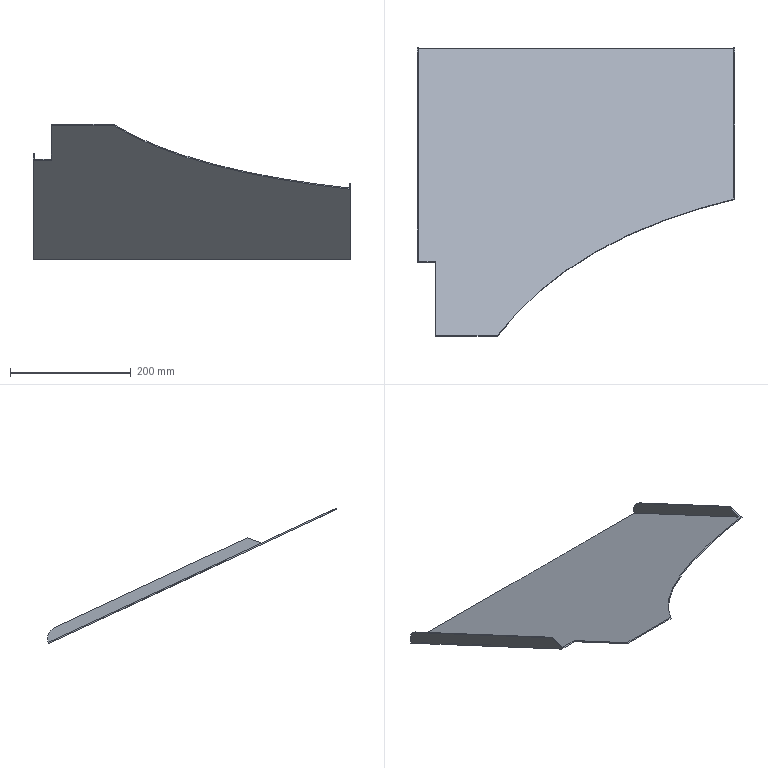Part | NX | features solid 2 | 1 solid | 17 faces | box 525 x 478.276 x 223.963 mm | volume 442323 mm3 | plane 14 | cylinder 2 | spline 1 | commonest cylinder face diameters 40 x2
STEP:
#1=CARTESIAN_POINT('',(-287.,720.,-282.15));
#2=VERTEX_POINT('',#1);
#3=CARTESIAN_POINT('',(-287.,720.,-279.943));
#4=VERTEX_POINT('',#3);
#5=CARTESIAN_POINT('',(-287.,720.,-430.));
#6=DIRECTION('',(0.,0.,1.));
#7=VECTOR('',#6,1000.);
#8=LINE('',#5,#7);
#9=EDGE_CURVE('',#2,#4,#8,.T.);
#10=ORIENTED_EDGE('',*,*,#9,.F.);
#11=CARTESIAN_POINT('',(-808.,720.,-282.15));
#12=VERTEX_POINT('',#11);
#13=CARTESIAN_POINT('',(188.564,720.,-282.15));
#14=DIRECTION('',(-1.,0.,0.));
#15=VECTOR('',#14,1000.);
#16=LINE('',#13,#15);
#17=EDGE_CURVE('',#2,#12,#16,.T.);
#18=ORIENTED_EDGE('',*,*,#17,.T.);
#19=CARTESIAN_POINT('',(-808.,720.,-279.943));
#20=VERTEX_POINT('',#19);
#21=CARTESIAN_POINT('',(-808.,720.,-430.));
#22=DIRECTION('',(0.,0.,-1.));
#23=VECTOR('',#22,1000.);
#24=LINE('',#21,#23);
#25=EDGE_CURVE('',#20,#12,#24,.T.);
#26=ORIENTED_EDGE('',*,*,#25,.F.);
#27=CARTESIAN_POINT('',(188.564,720.,-279.943));
#28=DIRECTION('',(-1.,0.,0.));
#29=VECTOR('',#28,1000.);
#30=LINE('',#27,#29);
#31=EDGE_CURVE('',#4,#20,#30,.T.);
#32=ORIENTED_EDGE('',*,*,#31,.F.);
#33=EDGE_LOOP('',(#10,#18,#26,#32));
#34=FACE_BOUND('',#33,.T.);
#35=CARTESIAN_POINT('',(188.564,720.,-430.));
#36=DIRECTION('',(0.,-1.,0.));
#37=DIRECTION('',(-1.,0.,0.));
#38=AXIS2_PLACEMENT_3D('',#35,#36,#37);
#39=PLANE('',#38);
#40=ADVANCED_FACE('',(#34),#39,.F.);
#41=CARTESIAN_POINT('',(-287.,472.974,-164.753));
#42=VERTEX_POINT('',#41);
#43=CARTESIAN_POINT('',(-285.,472.974,-164.753));
#44=VERTEX_POINT('',#43);
#45=CARTESIAN_POINT('',(-353.018,472.974,-164.753));
#46=DIRECTION('',(-1.,0.,0.));
#47=VECTOR('',#46,1000.);
#48=LINE('',#45,#47);
#49=EDGE_CURVE('',#42,#44,#48,.F.);
#50=ORIENTED_EDGE('',*,*,#49,.F.);
#51=CARTESIAN_POINT('',(-287.,417.055,-138.678));
#52=DIRECTION('',(0.,0.9063,-0.4226));
#53=VECTOR('',#52,1000.);
#54=LINE('',#51,#53);
#55=EDGE_CURVE('',#42,#4,#54,.T.);
#56=ORIENTED_EDGE('',*,*,#55,.T.);
#57=ORIENTED_EDGE('',*,*,#31,.T.);
#58=CARTESIAN_POINT('',(-808.,367.658,-115.644));
#59=VERTEX_POINT('',#58);
#60=CARTESIAN_POINT('',(-808.,417.055,-138.678));
#61=DIRECTION('',(0.,-0.9063,0.4226));
#62=VECTOR('',#61,1000.);
#63=LINE('',#60,#62);
#64=EDGE_CURVE('',#20,#59,#63,.T.);
#65=ORIENTED_EDGE('',*,*,#64,.T.);
#66=CARTESIAN_POINT('',(-780.,367.658,-115.644));
#67=VERTEX_POINT('',#66);
#68=CARTESIAN_POINT('',(-779.,367.658,-115.644));
#69=DIRECTION('',(-1.,0.,0.));
#70=VECTOR('',#69,1000.);
#71=LINE('',#68,#70);
#72=EDGE_CURVE('',#67,#59,#71,.T.);
#73=ORIENTED_EDGE('',*,*,#72,.F.);
#74=CARTESIAN_POINT('',(-780.,244.443,-58.187));
#75=VERTEX_POINT('',#74);
#76=CARTESIAN_POINT('',(-780.,272.567,-71.302));
#77=DIRECTION('',(0.,0.9063,-0.4226));
#78=VECTOR('',#77,1000.);
#79=LINE('',#76,#78);
#80=EDGE_CURVE('',#75,#67,#79,.T.);
#81=ORIENTED_EDGE('',*,*,#80,.F.);
#82=CARTESIAN_POINT('',(-677.72,244.443,-58.187));
#83=VERTEX_POINT('',#82);
#84=CARTESIAN_POINT('',(-353.018,244.443,-58.187));
#85=DIRECTION('',(1.,0.,0.));
#86=VECTOR('',#85,1000.);
#87=LINE('',#84,#86);
#88=EDGE_CURVE('',#75,#83,#87,.T.);
#89=ORIENTED_EDGE('',*,*,#88,.T.);
#90=CARTESIAN_POINT('',(-285.,471.162,-163.908));
#91=VERTEX_POINT('',#90);
#92=CARTESIAN_POINT('',(-677.72,244.443,-58.187));
#93=CARTESIAN_POINT('',(-672.167,251.77,-61.604));
#94=CARTESIAN_POINT('',(-663.423,262.605,-66.657));
#95=CARTESIAN_POINT('',(-650.978,276.698,-73.228));
#96=CARTESIAN_POINT('',(-641.165,287.179,-78.116));
#97=CARTESIAN_POINT('',(-631.216,297.219,-82.798));
#98=CARTESIAN_POINT('',(-620.962,307.004,-87.36));
#99=CARTESIAN_POINT('',(-612.158,314.946,-91.063));
#100=CARTESIAN_POINT('',(-604.955,321.177,-93.969));
#101=CARTESIAN_POINT('',(-600.401,325.008,-95.756));
#102=CARTESIAN_POINT('',(-596.688,328.067,-97.182));
#103=CARTESIAN_POINT('',(-593.065,331.011,-98.555));
#104=CARTESIAN_POINT('',(-586.789,336.01,-100.886));
#105=CARTESIAN_POINT('',(-573.857,345.914,-105.504));
#106=CARTESIAN_POINT('',(-558.47,356.808,-110.584));
#107=CARTESIAN_POINT('',(-542.419,367.323,-115.487));
#108=CARTESIAN_POINT('',(-530.057,375.012,-119.073));
#109=CARTESIAN_POINT('',(-517.377,382.503,-122.566));
#110=CARTESIAN_POINT('',(-506.516,388.595,-125.406));
#111=CARTESIAN_POINT('',(-498.82,392.748,-127.343));
#112=CARTESIAN_POINT('',(-494.304,395.136,-128.457));
#113=CARTESIAN_POINT('',(-490.241,397.26,-129.447));
#114=CARTESIAN_POINT('',(-484.961,399.97,-130.711));
#115=CARTESIAN_POINT('',(-476.523,404.197,-132.682));
#116=CARTESIAN_POINT('',(-465.791,409.379,-135.099));
#117=CARTESIAN_POINT('',(-448.313,417.413,-138.845));
#118=CARTESIAN_POINT('',(-430.339,425.076,-142.418));
#119=CARTESIAN_POINT('',(-411.886,432.361,-145.815));
#120=CARTESIAN_POINT('',(-400.134,436.764,-147.868));
#121=CARTESIAN_POINT('',(-390.645,440.181,-149.462));
#122=CARTESIAN_POINT('',(-383.373,442.729,-150.65));
#123=CARTESIAN_POINT('',(-376.401,445.108,-151.759));
#124=CARTESIAN_POINT('',(-367.079,448.209,-153.205));
#125=CARTESIAN_POINT('',(-357.741,451.192,-154.596));
#126=CARTESIAN_POINT('',(-348.382,454.06,-155.933));
#127=CARTESIAN_POINT('',(-341.353,456.153,-156.91));
#128=CARTESIAN_POINT('',(-335.488,457.849,-157.7));
#129=CARTESIAN_POINT('',(-330.79,459.178,-158.32));
#130=CARTESIAN_POINT('',(-327.855,459.995,-158.701));
#131=CARTESIAN_POINT('',(-325.793,460.562,-158.966));
#132=CARTESIAN_POINT('',(-324.625,460.882,-159.115));
#133=CARTESIAN_POINT('',(-323.869,461.088,-159.211));
#134=CARTESIAN_POINT('',(-323.323,461.236,-159.28));
#135=CARTESIAN_POINT('',(-322.949,461.338,-159.327));
#136=CARTESIAN_POINT('',(-322.199,461.541,-159.422));
#137=CARTESIAN_POINT('',(-320.706,461.943,-159.609));
#138=CARTESIAN_POINT('',(-318.393,462.561,-159.898));
#139=CARTESIAN_POINT('',(-314.394,463.619,-160.391));
#140=CARTESIAN_POINT('',(-308.795,465.082,-161.073));
#141=CARTESIAN_POINT('',(-302.405,466.73,-161.842));
#142=CARTESIAN_POINT('',(-297.517,467.981,-162.425));
#143=CARTESIAN_POINT('',(-294.603,468.725,-162.772));
#144=CARTESIAN_POINT('',(-292.74,469.199,-162.993));
#145=CARTESIAN_POINT('',(-291.2,469.59,-163.175));
#146=CARTESIAN_POINT('',(-290.27,469.826,-163.286));
#147=CARTESIAN_POINT('',(-289.417,470.043,-163.386));
#148=CARTESIAN_POINT('',(-288.93,470.166,-163.444));
#149=CARTESIAN_POINT('',(-287.978,470.408,-163.557));
#150=CARTESIAN_POINT('',(-286.649,470.744,-163.714));
#151=CARTESIAN_POINT('',(-285.552,471.022,-163.843));
#152=CARTESIAN_POINT('',(-285.,471.162,-163.908));
#153=B_SPLINE_CURVE_WITH_KNOTS('',3,(#92,#93,#94,#95,#96,#97,#98,#99,#100,#101,#102,#103,#104,#105,#106,#107,#108,#109,#110,#111,#112,#113,#114,#115,#116,#117,#118,#119,#120,#121,#122,#123,#124,#125,#126,#127,#128,#129,#130,#131,#132,#133,#134,#135,#136,#137,#138,#139,#140,#141,#142,#143,#144,#145,#146,#147,#148,#149,#150,#151,#152),.UNSPECIFIED.,.F.,.F.,(4,1,1,1,1,1,1,1,1,1,1,1,1,1,1,1,1,1,1,1,1,1,1,1,1,1,1,1,1,1,1,1,1,1,1,1,1,1,1,1,1,1,1,1,1,1,1,1,1,1,1,1,1,1,1,1,1,1,4),(0.,0.02989,0.04484,0.05979,0.07473,0.08968,0.1046,0.1121,0.1196,0.1233,0.127,0.1345,0.1495,0.1794,0.1943,0.2093,0.2242,0.2392,0.2466,0.2504,0.2541,0.2616,0.269,0.284,0.2989,0.3288,0.3438,0.3587,0.3662,0.3737,0.3811,0.3886,0.4036,0.411,0.4185,0.426,0.4297,0.4335,0.4353,0.4363,0.4372,0.4377,0.4381,0.4391,0.4409,0.4447,0.4484,0.4559,0.4634,0.4671,0.469,0.4708,0.4718,0.4727,0.4732,0.4736,0.4746,0.4764,0.4783),.UNSPECIFIED.);
#154=EDGE_CURVE('',#83,#91,#153,.T.);
#155=ORIENTED_EDGE('',*,*,#154,.T.);
#156=CARTESIAN_POINT('',(-285.,417.055,-138.678));
#157=DIRECTION('',(0.,0.9063,-0.4226));
#158=VECTOR('',#157,1000.);
#159=LINE('',#156,#158);
#160=EDGE_CURVE('',#91,#44,#159,.T.);
#161=ORIENTED_EDGE('',*,*,#160,.T.);
#162=EDGE_LOOP('',(#50,#56,#57,#65,#73,#81,#89,#155,#161));
#163=FACE_BOUND('',#162,.T.);
#164=CARTESIAN_POINT('',(-353.018,417.055,-138.678));
#165=DIRECTION('',(0.,0.4226,0.9063));
#166=DIRECTION('',(1.,0.,0.));
#167=AXIS2_PLACEMENT_3D('',#164,#165,#166);
#168=PLANE('',#167);
#169=ADVANCED_FACE('',(#163),#168,.T.);
#170=CARTESIAN_POINT('',(-285.,470.316,-165.721));
#171=VERTEX_POINT('',#170);
#172=CARTESIAN_POINT('',(-285.,471.162,-163.908));
#173=DIRECTION('',(0.,-0.4226,-0.9063));
#174=VECTOR('',#173,1000.);
#175=LINE('',#172,#174);
#176=EDGE_CURVE('',#91,#171,#175,.T.);
#177=ORIENTED_EDGE('',*,*,#176,.F.);
#178=ORIENTED_EDGE('',*,*,#154,.F.);
#179=CARTESIAN_POINT('',(-677.72,243.597,-60.));
#180=VERTEX_POINT('',#179);
#181=CARTESIAN_POINT('',(-677.72,243.597,-60.));
#182=CARTESIAN_POINT('',(-677.72,243.879,-59.396));
#183=CARTESIAN_POINT('',(-677.72,244.161,-58.792));
#184=CARTESIAN_POINT('',(-677.72,244.443,-58.187));
#185=B_SPLINE_CURVE_WITH_KNOTS('',3,(#181,#182,#183,#184),.UNSPECIFIED.,.F.,.F.,(4,4),(0.,1.),.UNSPECIFIED.);
#186=EDGE_CURVE('',#83,#180,#185,.F.);
#187=ORIENTED_EDGE('',*,*,#186,.T.);
#188=CARTESIAN_POINT('',(-677.72,243.597,-60.));
#189=CARTESIAN_POINT('',(-672.167,250.924,-63.417));
#190=CARTESIAN_POINT('',(-663.423,261.76,-68.469));
#191=CARTESIAN_POINT('',(-650.978,275.853,-75.041));
#192=CARTESIAN_POINT('',(-641.165,286.334,-79.928));
#193=CARTESIAN_POINT('',(-631.216,296.374,-84.61));
#194=CARTESIAN_POINT('',(-620.962,306.159,-89.173));
#195=CARTESIAN_POINT('',(-612.158,314.1,-92.876));
#196=CARTESIAN_POINT('',(-604.955,320.332,-95.782));
#197=CARTESIAN_POINT('',(-600.401,324.163,-97.568));
#198=CARTESIAN_POINT('',(-596.688,327.222,-98.995));
#199=CARTESIAN_POINT('',(-593.065,330.165,-100.367));
#200=CARTESIAN_POINT('',(-586.789,335.164,-102.698));
#201=CARTESIAN_POINT('',(-573.857,345.068,-107.317));
#202=CARTESIAN_POINT('',(-558.47,355.963,-112.397));
#203=CARTESIAN_POINT('',(-542.419,366.477,-117.3));
#204=CARTESIAN_POINT('',(-530.057,374.167,-120.886));
#205=CARTESIAN_POINT('',(-517.377,381.657,-124.378));
#206=CARTESIAN_POINT('',(-506.516,387.749,-127.219));
#207=CARTESIAN_POINT('',(-498.82,391.902,-129.156));
#208=CARTESIAN_POINT('',(-494.304,394.291,-130.27));
#209=CARTESIAN_POINT('',(-490.241,396.414,-131.26));
#210=CARTESIAN_POINT('',(-484.961,399.125,-132.524));
#211=CARTESIAN_POINT('',(-476.523,403.351,-134.494));
#212=CARTESIAN_POINT('',(-465.791,408.534,-136.911));
#213=CARTESIAN_POINT('',(-448.313,416.568,-140.657));
#214=CARTESIAN_POINT('',(-430.339,424.231,-144.231));
#215=CARTESIAN_POINT('',(-411.886,431.516,-147.628));
#216=CARTESIAN_POINT('',(-400.134,435.919,-149.681));
#217=CARTESIAN_POINT('',(-390.645,439.336,-151.274));
#218=CARTESIAN_POINT('',(-383.373,441.884,-152.463));
#219=CARTESIAN_POINT('',(-376.401,444.263,-153.572));
#220=CARTESIAN_POINT('',(-367.079,447.363,-155.018));
#221=CARTESIAN_POINT('',(-357.741,450.347,-156.409));
#222=CARTESIAN_POINT('',(-348.382,453.215,-157.746));
#223=CARTESIAN_POINT('',(-341.353,455.308,-158.722));
#224=CARTESIAN_POINT('',(-335.488,457.004,-159.513));
#225=CARTESIAN_POINT('',(-330.79,458.332,-160.133));
#226=CARTESIAN_POINT('',(-327.855,459.15,-160.514));
#227=CARTESIAN_POINT('',(-325.793,459.717,-160.778));
#228=CARTESIAN_POINT('',(-324.625,460.037,-160.927));
#229=CARTESIAN_POINT('',(-323.869,460.243,-161.023));
#230=CARTESIAN_POINT('',(-323.323,460.391,-161.093));
#231=CARTESIAN_POINT('',(-322.949,460.493,-161.14));
#232=CARTESIAN_POINT('',(-322.199,460.696,-161.235));
#233=CARTESIAN_POINT('',(-320.706,461.098,-161.422));
#234=CARTESIAN_POINT('',(-318.393,461.716,-161.71));
#235=CARTESIAN_POINT('',(-314.394,462.773,-162.203));
#236=CARTESIAN_POINT('',(-308.795,464.237,-162.886));
#237=CARTESIAN_POINT('',(-302.405,465.885,-163.654));
#238=CARTESIAN_POINT('',(-297.517,467.136,-164.238));
#239=CARTESIAN_POINT('',(-294.603,467.88,-164.584));
#240=CARTESIAN_POINT('',(-292.74,468.354,-164.806));
#241=CARTESIAN_POINT('',(-291.2,468.745,-164.988));
#242=CARTESIAN_POINT('',(-290.27,468.981,-165.098));
#243=CARTESIAN_POINT('',(-289.417,469.198,-165.199));
#244=CARTESIAN_POINT('',(-288.93,469.321,-165.257));
#245=CARTESIAN_POINT('',(-287.978,469.562,-165.369));
#246=CARTESIAN_POINT('',(-286.649,469.899,-165.526));
#247=CARTESIAN_POINT('',(-285.552,470.177,-165.656));
#248=CARTESIAN_POINT('',(-285.,470.316,-165.721));
#249=B_SPLINE_CURVE_WITH_KNOTS('',3,(#188,#189,#190,#191,#192,#193,#194,#195,#196,#197,#198,#199,#200,#201,#202,#203,#204,#205,#206,#207,#208,#209,#210,#211,#212,#213,#214,#215,#216,#217,#218,#219,#220,#221,#222,#223,#224,#225,#226,#227,#228,#229,#230,#231,#232,#233,#234,#235,#236,#237,#238,#239,#240,#241,#242,#243,#244,#245,#246,#247,#248),.UNSPECIFIED.,.F.,.F.,(4,1,1,1,1,1,1,1,1,1,1,1,1,1,1,1,1,1,1,1,1,1,1,1,1,1,1,1,1,1,1,1,1,1,1,1,1,1,1,1,1,1,1,1,1,1,1,1,1,1,1,1,1,1,1,1,1,1,4),(0.,0.02989,0.04484,0.05979,0.07473,0.08968,0.1046,0.1121,0.1196,0.1233,0.127,0.1345,0.1495,0.1794,0.1943,0.2093,0.2242,0.2392,0.2466,0.2504,0.2541,0.2616,0.269,0.284,0.2989,0.3288,0.3438,0.3587,0.3662,0.3737,0.3811,0.3886,0.4036,0.411,0.4185,0.426,0.4297,0.4335,0.4353,0.4363,0.4372,0.4377,0.4381,0.4391,0.4409,0.4447,0.4484,0.4559,0.4634,0.4671,0.469,0.4708,0.4718,0.4727,0.4732,0.4736,0.4746,0.4764,0.4783),.UNSPECIFIED.);
#250=EDGE_CURVE('',#180,#171,#249,.T.);
#251=ORIENTED_EDGE('',*,*,#250,.T.);
#252=EDGE_LOOP('',(#177,#178,#187,#251));
#253=FACE_BOUND('',#252,.T.);
#254=CARTESIAN_POINT('',(-677.72,244.443,-58.187));
#255=CARTESIAN_POINT('',(-677.72,243.597,-60.));
#256=CARTESIAN_POINT('',(-672.167,251.77,-61.604));
#257=CARTESIAN_POINT('',(-672.167,250.924,-63.417));
#258=CARTESIAN_POINT('',(-663.423,262.605,-66.657));
#259=CARTESIAN_POINT('',(-663.423,261.76,-68.469));
#260=CARTESIAN_POINT('',(-650.978,276.698,-73.228));
#261=CARTESIAN_POINT('',(-650.978,275.853,-75.041));
#262=CARTESIAN_POINT('',(-641.165,287.179,-78.116));
#263=CARTESIAN_POINT('',(-641.165,286.334,-79.928));
#264=CARTESIAN_POINT('',(-631.216,297.219,-82.798));
#265=CARTESIAN_POINT('',(-631.216,296.374,-84.61));
#266=CARTESIAN_POINT('',(-620.962,307.004,-87.36));
#267=CARTESIAN_POINT('',(-620.962,306.159,-89.173));
#268=CARTESIAN_POINT('',(-612.158,314.946,-91.063));
#269=CARTESIAN_POINT('',(-612.158,314.1,-92.876));
#270=CARTESIAN_POINT('',(-604.955,321.177,-93.969));
#271=CARTESIAN_POINT('',(-604.955,320.332,-95.782));
#272=CARTESIAN_POINT('',(-600.401,325.008,-95.756));
#273=CARTESIAN_POINT('',(-600.401,324.163,-97.568));
#274=CARTESIAN_POINT('',(-596.688,328.067,-97.182));
#275=CARTESIAN_POINT('',(-596.688,327.222,-98.995));
#276=CARTESIAN_POINT('',(-593.065,331.011,-98.555));
#277=CARTESIAN_POINT('',(-593.065,330.165,-100.367));
#278=CARTESIAN_POINT('',(-586.789,336.01,-100.886));
#279=CARTESIAN_POINT('',(-586.789,335.164,-102.698));
#280=CARTESIAN_POINT('',(-573.857,345.914,-105.504));
#281=CARTESIAN_POINT('',(-573.857,345.068,-107.317));
#282=CARTESIAN_POINT('',(-558.47,356.808,-110.584));
#283=CARTESIAN_POINT('',(-558.47,355.963,-112.397));
#284=CARTESIAN_POINT('',(-542.419,367.323,-115.487));
#285=CARTESIAN_POINT('',(-542.419,366.477,-117.3));
#286=CARTESIAN_POINT('',(-530.057,375.012,-119.073));
#287=CARTESIAN_POINT('',(-530.057,374.167,-120.886));
#288=CARTESIAN_POINT('',(-517.377,382.503,-122.566));
#289=CARTESIAN_POINT('',(-517.377,381.657,-124.378));
#290=CARTESIAN_POINT('',(-506.516,388.595,-125.406));
#291=CARTESIAN_POINT('',(-506.516,387.749,-127.219));
#292=CARTESIAN_POINT('',(-498.82,392.748,-127.343));
#293=CARTESIAN_POINT('',(-498.82,391.902,-129.156));
#294=CARTESIAN_POINT('',(-494.304,395.136,-128.457));
#295=CARTESIAN_POINT('',(-494.304,394.291,-130.27));
#296=CARTESIAN_POINT('',(-490.241,397.26,-129.447));
#297=CARTESIAN_POINT('',(-490.241,396.414,-131.26));
#298=CARTESIAN_POINT('',(-484.961,399.97,-130.711));
#299=CARTESIAN_POINT('',(-484.961,399.125,-132.524));
#300=CARTESIAN_POINT('',(-476.523,404.197,-132.682));
#301=CARTESIAN_POINT('',(-476.523,403.351,-134.494));
#302=CARTESIAN_POINT('',(-465.791,409.379,-135.099));
#303=CARTESIAN_POINT('',(-465.791,408.534,-136.911));
#304=CARTESIAN_POINT('',(-448.313,417.413,-138.845));
#305=CARTESIAN_POINT('',(-448.313,416.568,-140.657));
#306=CARTESIAN_POINT('',(-430.339,425.076,-142.418));
#307=CARTESIAN_POINT('',(-430.339,424.231,-144.231));
#308=CARTESIAN_POINT('',(-411.886,432.361,-145.815));
#309=CARTESIAN_POINT('',(-411.886,431.516,-147.628));
#310=CARTESIAN_POINT('',(-400.134,436.764,-147.868));
#311=CARTESIAN_POINT('',(-400.134,435.919,-149.681));
#312=CARTESIAN_POINT('',(-390.645,440.181,-149.462));
#313=CARTESIAN_POINT('',(-390.645,439.336,-151.274));
#314=CARTESIAN_POINT('',(-383.373,442.729,-150.65));
#315=CARTESIAN_POINT('',(-383.373,441.884,-152.463));
#316=CARTESIAN_POINT('',(-376.401,445.108,-151.759));
#317=CARTESIAN_POINT('',(-376.401,444.263,-153.572));
#318=CARTESIAN_POINT('',(-367.079,448.209,-153.205));
#319=CARTESIAN_POINT('',(-367.079,447.363,-155.018));
#320=CARTESIAN_POINT('',(-357.741,451.192,-154.596));
#321=CARTESIAN_POINT('',(-357.741,450.347,-156.409));
#322=CARTESIAN_POINT('',(-348.382,454.06,-155.933));
#323=CARTESIAN_POINT('',(-348.382,453.215,-157.746));
#324=CARTESIAN_POINT('',(-341.353,456.153,-156.91));
#325=CARTESIAN_POINT('',(-341.353,455.308,-158.722));
#326=CARTESIAN_POINT('',(-335.488,457.849,-157.7));
#327=CARTESIAN_POINT('',(-335.488,457.004,-159.513));
#328=CARTESIAN_POINT('',(-330.79,459.178,-158.32));
#329=CARTESIAN_POINT('',(-330.79,458.332,-160.133));
#330=CARTESIAN_POINT('',(-327.855,459.995,-158.701));
#331=CARTESIAN_POINT('',(-327.855,459.15,-160.514));
#332=CARTESIAN_POINT('',(-325.793,460.562,-158.966));
#333=CARTESIAN_POINT('',(-325.793,459.717,-160.778));
#334=CARTESIAN_POINT('',(-324.625,460.882,-159.115));
#335=CARTESIAN_POINT('',(-324.625,460.037,-160.927));
#336=CARTESIAN_POINT('',(-323.869,461.088,-159.211));
#337=CARTESIAN_POINT('',(-323.869,460.243,-161.023));
#338=CARTESIAN_POINT('',(-323.323,461.236,-159.28));
#339=CARTESIAN_POINT('',(-323.323,460.391,-161.093));
#340=CARTESIAN_POINT('',(-322.949,461.338,-159.327));
#341=CARTESIAN_POINT('',(-322.949,460.493,-161.14));
#342=CARTESIAN_POINT('',(-322.199,461.541,-159.422));
#343=CARTESIAN_POINT('',(-322.199,460.696,-161.235));
#344=CARTESIAN_POINT('',(-320.706,461.943,-159.609));
#345=CARTESIAN_POINT('',(-320.706,461.098,-161.422));
#346=CARTESIAN_POINT('',(-318.393,462.561,-159.898));
#347=CARTESIAN_POINT('',(-318.393,461.716,-161.71));
#348=CARTESIAN_POINT('',(-314.394,463.619,-160.391));
#349=CARTESIAN_POINT('',(-314.394,462.773,-162.203));
#350=CARTESIAN_POINT('',(-308.795,465.082,-161.073));
#351=CARTESIAN_POINT('',(-308.795,464.237,-162.886));
#352=CARTESIAN_POINT('',(-302.405,466.73,-161.842));
#353=CARTESIAN_POINT('',(-302.405,465.885,-163.654));
#354=CARTESIAN_POINT('',(-297.517,467.981,-162.425));
#355=CARTESIAN_POINT('',(-297.517,467.136,-164.238));
#356=CARTESIAN_POINT('',(-294.603,468.725,-162.772));
#357=CARTESIAN_POINT('',(-294.603,467.88,-164.584));
#358=CARTESIAN_POINT('',(-292.74,469.199,-162.993));
#359=CARTESIAN_POINT('',(-292.74,468.354,-164.806));
#360=CARTESIAN_POINT('',(-291.2,469.59,-163.175));
#361=CARTESIAN_POINT('',(-291.2,468.745,-164.988));
#362=CARTESIAN_POINT('',(-290.27,469.826,-163.286));
#363=CARTESIAN_POINT('',(-290.27,468.981,-165.098));
#364=CARTESIAN_POINT('',(-289.417,470.043,-163.386));
#365=CARTESIAN_POINT('',(-289.417,469.198,-165.199));
#366=CARTESIAN_POINT('',(-288.93,470.166,-163.444));
#367=CARTESIAN_POINT('',(-288.93,469.321,-165.257));
#368=CARTESIAN_POINT('',(-287.978,470.408,-163.557));
#369=CARTESIAN_POINT('',(-287.978,469.562,-165.369));
#370=CARTESIAN_POINT('',(-286.649,470.744,-163.714));
#371=CARTESIAN_POINT('',(-286.649,469.899,-165.526));
#372=CARTESIAN_POINT('',(-285.552,471.022,-163.843));
#373=CARTESIAN_POINT('',(-285.552,470.177,-165.656));
#374=CARTESIAN_POINT('',(-285.,471.162,-163.908));
#375=CARTESIAN_POINT('',(-285.,470.316,-165.721));
#376=B_SPLINE_SURFACE_WITH_KNOTS('',3,1,((#254,#255),(#256,#257),(#258,#259),(#260,#261),(#262,#263),(#264,#265),(#266,#267),(#268,#269),(#270,#271),(#272,#273),(#274,#275),(#276,#277),(#278,#279),(#280,#281),(#282,#283),(#284,#285),(#286,#287),(#288,#289),(#290,#291),(#292,#293),(#294,#295),(#296,#297),(#298,#299),(#300,#301),(#302,#303),(#304,#305),(#306,#307),(#308,#309),(#310,#311),(#312,#313),(#314,#315),(#316,#317),(#318,#319),(#320,#321),(#322,#323),(#324,#325),(#326,#327),(#328,#329),(#330,#331),(#332,#333),(#334,#335),(#336,#337),(#338,#339),(#340,#341),(#342,#343),(#344,#345),(#346,#347),(#348,#349),(#350,#351),(#352,#353),(#354,#355),(#356,#357),(#358,#359),(#360,#361),(#362,#363),(#364,#365),(#366,#367),(#368,#369),(#370,#371),(#372,#373),(#374,#375)),.SURF_OF_LINEAR_EXTRUSION.,.F.,.F.,.F.,(4,1,1,1,1,1,1,1,1,1,1,1,1,1,1,1,1,1,1,1,1,1,1,1,1,1,1,1,1,1,1,1,1,1,1,1,1,1,1,1,1,1,1,1,1,1,1,1,1,1,1,1,1,1,1,1,1,1,4),(2,2),(0.,0.02989,0.04484,0.05979,0.07473,0.08968,0.1046,0.1121,0.1196,0.1233,0.127,0.1345,0.1495,0.1794,0.1943,0.2093,0.2242,0.2392,0.2466,0.2504,0.2541,0.2616,0.269,0.284,0.2989,0.3288,0.3438,0.3587,0.3662,0.3737,0.3811,0.3886,0.4036,0.411,0.4185,0.426,0.4297,0.4335,0.4353,0.4363,0.4372,0.4377,0.4381,0.4391,0.4409,0.4447,0.4484,0.4559,0.4634,0.4671,0.469,0.4708,0.4718,0.4727,0.4732,0.4736,0.4746,0.4764,0.4783),(0.,1.),.UNSPECIFIED.);
#377=ADVANCED_FACE('',(#253),#376,.F.);
#378=ORIENTED_EDGE('',*,*,#17,.F.);
#379=CARTESIAN_POINT('',(-285.,720.,-282.15));
#380=VERTEX_POINT('',#379);
#381=CARTESIAN_POINT('',(188.564,720.,-282.15));
#382=DIRECTION('',(-1.,0.,0.));
#383=VECTOR('',#382,1000.);
#384=LINE('',#381,#383);
#385=EDGE_CURVE('',#380,#2,#384,.T.);
#386=ORIENTED_EDGE('',*,*,#385,.F.);
#387=CARTESIAN_POINT('',(-285.,416.21,-140.491));
#388=DIRECTION('',(0.,0.9063,-0.4226));
#389=VECTOR('',#388,1000.);
#390=LINE('',#387,#389);
#391=EDGE_CURVE('',#171,#380,#390,.T.);
#392=ORIENTED_EDGE('',*,*,#391,.F.);
#393=ORIENTED_EDGE('',*,*,#250,.F.);
#394=CARTESIAN_POINT('',(-780.,243.597,-60.));
#395=VERTEX_POINT('',#394);
#396=CARTESIAN_POINT('',(-353.018,243.597,-60.));
#397=DIRECTION('',(1.,0.,0.));
#398=VECTOR('',#397,1000.);
#399=LINE('',#396,#398);
#400=EDGE_CURVE('',#395,#180,#399,.T.);
#401=ORIENTED_EDGE('',*,*,#400,.F.);
#402=CARTESIAN_POINT('',(-780.,366.813,-117.456));
#403=VERTEX_POINT('',#402);
#404=CARTESIAN_POINT('',(-780.,271.722,-73.114));
#405=DIRECTION('',(0.,0.9063,-0.4226));
#406=VECTOR('',#405,1000.);
#407=LINE('',#404,#406);
#408=EDGE_CURVE('',#395,#403,#407,.T.);
#409=ORIENTED_EDGE('',*,*,#408,.T.);
#410=CARTESIAN_POINT('',(-810.,366.813,-117.456));
#411=VERTEX_POINT('',#410);
#412=CARTESIAN_POINT('',(-779.,366.813,-117.456));
#413=DIRECTION('',(-1.,0.,0.));
#414=VECTOR('',#413,1000.);
#415=LINE('',#412,#414);
#416=EDGE_CURVE('',#403,#411,#415,.T.);
#417=ORIENTED_EDGE('',*,*,#416,.T.);
#418=CARTESIAN_POINT('',(-810.,720.,-282.15));
#419=VERTEX_POINT('',#418);
#420=CARTESIAN_POINT('',(-810.,559.597,-207.353));
#421=DIRECTION('',(0.,-0.9063,0.4226));
#422=VECTOR('',#421,1000.);
#423=LINE('',#420,#422);
#424=EDGE_CURVE('',#419,#411,#423,.T.);
#425=ORIENTED_EDGE('',*,*,#424,.F.);
#426=CARTESIAN_POINT('',(-800.,720.,-282.15));
#427=DIRECTION('',(1.,0.,0.));
#428=VECTOR('',#427,1000.);
#429=LINE('',#426,#428);
#430=EDGE_CURVE('',#419,#12,#429,.T.);
#431=ORIENTED_EDGE('',*,*,#430,.T.);
#432=EDGE_LOOP('',(#378,#386,#392,#393,#401,#409,#417,#425,#431));
#433=FACE_BOUND('',#432,.T.);
#434=CARTESIAN_POINT('',(-353.018,416.21,-140.491));
#435=DIRECTION('',(0.,0.4226,0.9063));
#436=DIRECTION('',(1.,0.,0.));
#437=AXIS2_PLACEMENT_3D('',#434,#435,#436);
#438=PLANE('',#437);
#439=ADVANCED_FACE('',(#433),#438,.F.);
#440=ORIENTED_EDGE('',*,*,#72,.T.);
#441=CARTESIAN_POINT('',(-810.,367.658,-115.644));
#442=VERTEX_POINT('',#441);
#443=CARTESIAN_POINT('',(-779.,367.658,-115.644));
#444=DIRECTION('',(-1.,0.,0.));
#445=VECTOR('',#444,1000.);
#446=LINE('',#443,#445);
#447=EDGE_CURVE('',#59,#442,#446,.T.);
#448=ORIENTED_EDGE('',*,*,#447,.T.);
#449=CARTESIAN_POINT('',(-810.,367.658,-115.644));
#450=DIRECTION('',(0.,-0.4226,-0.9063));
#451=VECTOR('',#450,1000.);
#452=LINE('',#449,#451);
#453=EDGE_CURVE('',#442,#411,#452,.T.);
#454=ORIENTED_EDGE('',*,*,#453,.T.);
#455=ORIENTED_EDGE('',*,*,#416,.F.);
#456=CARTESIAN_POINT('',(-780.,367.658,-115.644));
#457=DIRECTION('',(0.,-0.4226,-0.9063));
#458=VECTOR('',#457,1000.);
#459=LINE('',#456,#458);
#460=EDGE_CURVE('',#67,#403,#459,.T.);
#461=ORIENTED_EDGE('',*,*,#460,.F.);
#462=EDGE_LOOP('',(#440,#448,#454,#455,#461));
#463=FACE_BOUND('',#462,.T.);
#464=CARTESIAN_POINT('',(-779.,367.658,-115.644));
#465=DIRECTION('',(0.,-0.9063,0.4226));
#466=DIRECTION('',(0.,-0.4226,-0.9063));
#467=AXIS2_PLACEMENT_3D('',#464,#465,#466);
#468=PLANE('',#467);
#469=ADVANCED_FACE('',(#463),#468,.T.);
#470=ORIENTED_EDGE('',*,*,#408,.F.);
#471=CARTESIAN_POINT('',(-780.,244.443,-58.187));
#472=DIRECTION('',(0.,0.4226,0.9063));
#473=VECTOR('',#472,1000.);
#474=LINE('',#471,#473);
#475=EDGE_CURVE('',#395,#75,#474,.T.);
#476=ORIENTED_EDGE('',*,*,#475,.T.);
#477=ORIENTED_EDGE('',*,*,#80,.T.);
#478=ORIENTED_EDGE('',*,*,#460,.T.);
#479=EDGE_LOOP('',(#470,#476,#477,#478));
#480=FACE_BOUND('',#479,.T.);
#481=CARTESIAN_POINT('',(-780.,272.567,-71.302));
#482=DIRECTION('',(-1.,0.,0.));
#483=DIRECTION('',(0.,0.,1.));
#484=AXIS2_PLACEMENT_3D('',#481,#482,#483);
#485=PLANE('',#484);
#486=ADVANCED_FACE('',(#480),#485,.T.);
#487=ORIENTED_EDGE('',*,*,#475,.F.);
#488=ORIENTED_EDGE('',*,*,#400,.T.);
#489=ORIENTED_EDGE('',*,*,#186,.F.);
#490=ORIENTED_EDGE('',*,*,#88,.F.);
#491=EDGE_LOOP('',(#487,#488,#489,#490));
#492=FACE_BOUND('',#491,.T.);
#493=CARTESIAN_POINT('',(-353.018,244.443,-58.187));
#494=DIRECTION('',(0.,0.9063,-0.4226));
#495=DIRECTION('',(0.,0.4226,0.9063));
#496=AXIS2_PLACEMENT_3D('',#493,#494,#495);
#497=PLANE('',#496);
#498=ADVANCED_FACE('',(#492),#497,.F.);
#499=ORIENTED_EDGE('',*,*,#453,.F.);
#500=CARTESIAN_POINT('',(-810.,391.579,-106.937));
#501=VERTEX_POINT('',#500);
#502=CARTESIAN_POINT('',(-810.,367.658,-115.644));
#503=DIRECTION('',(0.,0.9397,0.342));
#504=VECTOR('',#503,1000.);
#505=LINE('',#502,#504);
#506=EDGE_CURVE('',#442,#501,#505,.T.);
#507=ORIENTED_EDGE('',*,*,#506,.T.);
#508=CARTESIAN_POINT('',(-810.,710.326,-255.572));
#509=VERTEX_POINT('',#508);
#510=CARTESIAN_POINT('',(-810.,568.049,-189.227));
#511=DIRECTION('',(0.,0.9063,-0.4226));
#512=VECTOR('',#511,1000.);
#513=LINE('',#510,#512);
#514=EDGE_CURVE('',#509,#501,#513,.F.);
#515=ORIENTED_EDGE('',*,*,#514,.F.);
#516=CARTESIAN_POINT('',(-810.,701.874,-273.698));
#517=DIRECTION('',(1.,0.,0.));
#518=DIRECTION('',(0.,0.,-1.));
#519=AXIS2_PLACEMENT_3D('',#516,#517,#518);
#520=CIRCLE('',#519,20.);
#521=EDGE_CURVE('',#509,#419,#520,.F.);
#522=ORIENTED_EDGE('',*,*,#521,.T.);
#523=ORIENTED_EDGE('',*,*,#424,.T.);
#524=EDGE_LOOP('',(#499,#507,#515,#522,#523));
#525=FACE_BOUND('',#524,.T.);
#526=CARTESIAN_POINT('',(-810.,560.442,-205.54));
#527=DIRECTION('',(1.,0.,0.));
#528=DIRECTION('',(0.,0.,-1.));
#529=AXIS2_PLACEMENT_3D('',#526,#527,#528);
#530=PLANE('',#529);
#531=ADVANCED_FACE('',(#525),#530,.F.);
#532=CARTESIAN_POINT('',(-808.,710.326,-255.572));
#533=VERTEX_POINT('',#532);
#534=CARTESIAN_POINT('',(-808.,391.579,-106.937));
#535=VERTEX_POINT('',#534);
#536=CARTESIAN_POINT('',(-808.,728.452,-264.024));
#537=DIRECTION('',(0.,0.9063,-0.4226));
#538=VECTOR('',#537,1000.);
#539=LINE('',#536,#538);
#540=EDGE_CURVE('',#533,#535,#539,.F.);
#541=ORIENTED_EDGE('',*,*,#540,.T.);
#542=CARTESIAN_POINT('',(-808.,367.658,-115.644));
#543=DIRECTION('',(0.,-0.9397,-0.342));
#544=VECTOR('',#543,1000.);
#545=LINE('',#542,#544);
#546=EDGE_CURVE('',#535,#59,#545,.T.);
#547=ORIENTED_EDGE('',*,*,#546,.T.);
#548=ORIENTED_EDGE('',*,*,#64,.F.);
#549=ORIENTED_EDGE('',*,*,#25,.T.);
#550=CARTESIAN_POINT('',(-808.,701.874,-273.698));
#551=DIRECTION('',(-1.,0.,0.));
#552=DIRECTION('',(0.,0.,1.));
#553=AXIS2_PLACEMENT_3D('',#550,#551,#552);
#554=CIRCLE('',#553,20.);
#555=EDGE_CURVE('',#12,#533,#554,.F.);
#556=ORIENTED_EDGE('',*,*,#555,.T.);
#557=EDGE_LOOP('',(#541,#547,#548,#549,#556));
#558=FACE_BOUND('',#557,.T.);
#559=CARTESIAN_POINT('',(-808.,720.,-282.15));
#560=DIRECTION('',(-1.,0.,0.));
#561=DIRECTION('',(0.,0.,1.));
#562=AXIS2_PLACEMENT_3D('',#559,#560,#561);
#563=PLANE('',#562);
#564=ADVANCED_FACE('',(#558),#563,.F.);
#565=ORIENTED_EDGE('',*,*,#514,.T.);
#566=CARTESIAN_POINT('',(-800.,391.579,-106.937));
#567=DIRECTION('',(-1.,0.,0.));
#568=VECTOR('',#567,1000.);
#569=LINE('',#566,#568);
#570=EDGE_CURVE('',#501,#535,#569,.F.);
#571=ORIENTED_EDGE('',*,*,#570,.T.);
#572=ORIENTED_EDGE('',*,*,#540,.F.);
#573=CARTESIAN_POINT('',(-800.,710.326,-255.572));
#574=DIRECTION('',(-1.,0.,0.));
#575=VECTOR('',#574,1000.);
#576=LINE('',#573,#575);
#577=EDGE_CURVE('',#533,#509,#576,.T.);
#578=ORIENTED_EDGE('',*,*,#577,.T.);
#579=EDGE_LOOP('',(#565,#571,#572,#578));
#580=FACE_BOUND('',#579,.T.);
#581=CARTESIAN_POINT('',(-800.,728.452,-264.024));
#582=DIRECTION('',(0.,-0.4226,-0.9063));
#583=DIRECTION('',(0.,-0.9063,0.4226));
#584=AXIS2_PLACEMENT_3D('',#581,#582,#583);
#585=PLANE('',#584);
#586=ADVANCED_FACE('',(#580),#585,.F.);
#587=ORIENTED_EDGE('',*,*,#521,.F.);
#588=ORIENTED_EDGE('',*,*,#577,.F.);
#589=ORIENTED_EDGE('',*,*,#555,.F.);
#590=ORIENTED_EDGE('',*,*,#430,.F.);
#591=EDGE_LOOP('',(#587,#588,#589,#590));
#592=FACE_BOUND('',#591,.T.);
#593=CARTESIAN_POINT('',(-800.,701.874,-273.698));
#594=DIRECTION('',(1.,0.,0.));
#595=DIRECTION('',(0.,0.,-1.));
#596=AXIS2_PLACEMENT_3D('',#593,#594,#595);
#597=CYLINDRICAL_SURFACE('',#596,20.);
#598=ADVANCED_FACE('',(#592),#597,.T.);
#599=ORIENTED_EDGE('',*,*,#176,.T.);
#600=ORIENTED_EDGE('',*,*,#391,.T.);
#601=CARTESIAN_POINT('',(-285.,710.326,-255.572));
#602=VERTEX_POINT('',#601);
#603=CARTESIAN_POINT('',(-285.,701.874,-273.698));
#604=DIRECTION('',(1.,0.,0.));
#605=DIRECTION('',(0.,0.,-1.));
#606=AXIS2_PLACEMENT_3D('',#603,#604,#605);
#607=CIRCLE('',#606,20.);
#608=EDGE_CURVE('',#380,#602,#607,.T.);
#609=ORIENTED_EDGE('',*,*,#608,.T.);
#610=CARTESIAN_POINT('',(-285.,496.895,-156.047));
#611=VERTEX_POINT('',#610);
#612=CARTESIAN_POINT('',(-285.,478.769,-147.595));
#613=DIRECTION('',(0.,0.9063,-0.4226));
#614=VECTOR('',#613,1000.);
#615=LINE('',#612,#614);
#616=EDGE_CURVE('',#611,#602,#615,.T.);
#617=ORIENTED_EDGE('',*,*,#616,.F.);
#618=CARTESIAN_POINT('',(-285.,470.316,-165.721));
#619=DIRECTION('',(0.,0.9397,0.342));
#620=VECTOR('',#619,1000.);
#621=LINE('',#618,#620);
#622=EDGE_CURVE('',#611,#44,#621,.F.);
#623=ORIENTED_EDGE('',*,*,#622,.T.);
#624=ORIENTED_EDGE('',*,*,#160,.F.);
#625=EDGE_LOOP('',(#599,#600,#609,#617,#623,#624));
#626=FACE_BOUND('',#625,.T.);
#627=CARTESIAN_POINT('',(-285.,610.,-55.));
#628=DIRECTION('',(1.,0.,0.));
#629=DIRECTION('',(0.,0.,-1.));
#630=AXIS2_PLACEMENT_3D('',#627,#628,#629);
#631=PLANE('',#630);
#632=ADVANCED_FACE('',(#626),#631,.T.);
#633=CARTESIAN_POINT('',(-287.,710.326,-255.572));
#634=VERTEX_POINT('',#633);
#635=CARTESIAN_POINT('',(-287.,701.874,-273.698));
#636=DIRECTION('',(1.,0.,0.));
#637=DIRECTION('',(0.,0.,-1.));
#638=AXIS2_PLACEMENT_3D('',#635,#636,#637);
#639=CIRCLE('',#638,20.);
#640=EDGE_CURVE('',#634,#2,#639,.F.);
#641=ORIENTED_EDGE('',*,*,#640,.T.);
#642=ORIENTED_EDGE('',*,*,#9,.T.);
#643=ORIENTED_EDGE('',*,*,#55,.F.);
#644=CARTESIAN_POINT('',(-287.,496.895,-156.047));
#645=VERTEX_POINT('',#644);
#646=CARTESIAN_POINT('',(-287.,470.316,-165.721));
#647=DIRECTION('',(0.,-0.9397,-0.342));
#648=VECTOR('',#647,1000.);
#649=LINE('',#646,#648);
#650=EDGE_CURVE('',#42,#645,#649,.F.);
#651=ORIENTED_EDGE('',*,*,#650,.T.);
#652=CARTESIAN_POINT('',(-287.,478.769,-147.595));
#653=DIRECTION('',(0.,0.9063,-0.4226));
#654=VECTOR('',#653,1000.);
#655=LINE('',#652,#654);
#656=EDGE_CURVE('',#645,#634,#655,.T.);
#657=ORIENTED_EDGE('',*,*,#656,.T.);
#658=EDGE_LOOP('',(#641,#642,#643,#651,#657));
#659=FACE_BOUND('',#658,.T.);
#660=CARTESIAN_POINT('',(-287.,470.316,-165.721));
#661=DIRECTION('',(1.,0.,0.));
#662=DIRECTION('',(0.,0.,-1.));
#663=AXIS2_PLACEMENT_3D('',#660,#661,#662);
#664=PLANE('',#663);
#665=ADVANCED_FACE('',(#659),#664,.F.);
#666=ORIENTED_EDGE('',*,*,#616,.T.);
#667=CARTESIAN_POINT('',(-285.,710.326,-255.572));
#668=DIRECTION('',(1.,0.,0.));
#669=VECTOR('',#668,1000.);
#670=LINE('',#667,#669);
#671=EDGE_CURVE('',#602,#634,#670,.F.);
#672=ORIENTED_EDGE('',*,*,#671,.T.);
#673=ORIENTED_EDGE('',*,*,#656,.F.);
#674=CARTESIAN_POINT('',(-285.,496.895,-156.047));
#675=DIRECTION('',(1.,0.,0.));
#676=VECTOR('',#675,1000.);
#677=LINE('',#674,#676);
#678=EDGE_CURVE('',#645,#611,#677,.T.);
#679=ORIENTED_EDGE('',*,*,#678,.T.);
#680=EDGE_LOOP('',(#666,#672,#673,#679));
#681=FACE_BOUND('',#680,.T.);
#682=CARTESIAN_POINT('',(-285.,478.769,-147.595));
#683=DIRECTION('',(0.,-0.4226,-0.9063));
#684=DIRECTION('',(0.,0.9063,-0.4226));
#685=AXIS2_PLACEMENT_3D('',#682,#683,#684);
#686=PLANE('',#685);
#687=ADVANCED_FACE('',(#681),#686,.F.);
#688=ORIENTED_EDGE('',*,*,#650,.F.);
#689=ORIENTED_EDGE('',*,*,#49,.T.);
#690=ORIENTED_EDGE('',*,*,#622,.F.);
#691=ORIENTED_EDGE('',*,*,#678,.F.);
#692=EDGE_LOOP('',(#688,#689,#690,#691));
#693=FACE_BOUND('',#692,.T.);
#694=CARTESIAN_POINT('',(-285.,470.316,-165.721));
#695=DIRECTION('',(0.,0.342,-0.9397));
#696=DIRECTION('',(0.,0.9397,0.342));
#697=AXIS2_PLACEMENT_3D('',#694,#695,#696);
#698=PLANE('',#697);
#699=ADVANCED_FACE('',(#693),#698,.F.);
#700=ORIENTED_EDGE('',*,*,#608,.F.);
#701=ORIENTED_EDGE('',*,*,#385,.T.);
#702=ORIENTED_EDGE('',*,*,#640,.F.);
#703=ORIENTED_EDGE('',*,*,#671,.F.);
#704=EDGE_LOOP('',(#700,#701,#702,#703));
#705=FACE_BOUND('',#704,.T.);
#706=CARTESIAN_POINT('',(-285.,701.874,-273.698));
#707=DIRECTION('',(1.,0.,0.));
#708=DIRECTION('',(0.,0.,-1.));
#709=AXIS2_PLACEMENT_3D('',#706,#707,#708);
#710=CYLINDRICAL_SURFACE('',#709,20.);
#711=ADVANCED_FACE('',(#705),#710,.T.);
#712=ORIENTED_EDGE('',*,*,#546,.F.);
#713=ORIENTED_EDGE('',*,*,#570,.F.);
#714=ORIENTED_EDGE('',*,*,#506,.F.);
#715=ORIENTED_EDGE('',*,*,#447,.F.);
#716=EDGE_LOOP('',(#712,#713,#714,#715));
#717=FACE_BOUND('',#716,.T.);
#718=CARTESIAN_POINT('',(-779.,367.658,-115.644));
#719=DIRECTION('',(0.,-0.342,0.9397));
#720=DIRECTION('',(0.,-0.9397,-0.342));
#721=AXIS2_PLACEMENT_3D('',#718,#719,#720);
#722=PLANE('',#721);
#723=ADVANCED_FACE('',(#717),#722,.T.);
#724=CLOSED_SHELL('',(#40,#169,#377,#439,#469,#486,#498,#531,#564,#586,#598,#632,#665,#687,#699,#711,#723));
#725=MANIFOLD_SOLID_BREP('',#724);
#726=(LENGTH_UNIT()NAMED_UNIT(*)SI_UNIT(.MILLI.,.METRE.));
#727=UNCERTAINTY_MEASURE_WITH_UNIT(LENGTH_MEASURE(0.0508),#726,'','');
#728=(NAMED_UNIT(*)PLANE_ANGLE_UNIT()SI_UNIT($,.RADIAN.));
#729=(NAMED_UNIT(*)SI_UNIT($,.STERADIAN.)SOLID_ANGLE_UNIT());
#730=(GEOMETRIC_REPRESENTATION_CONTEXT(3)GLOBAL_UNCERTAINTY_ASSIGNED_CONTEXT((#727))GLOBAL_UNIT_ASSIGNED_CONTEXT((#726,#728,#729))REPRESENTATION_CONTEXT('',''));
#731=ADVANCED_BREP_SHAPE_REPRESENTATION('',(#725),#730);